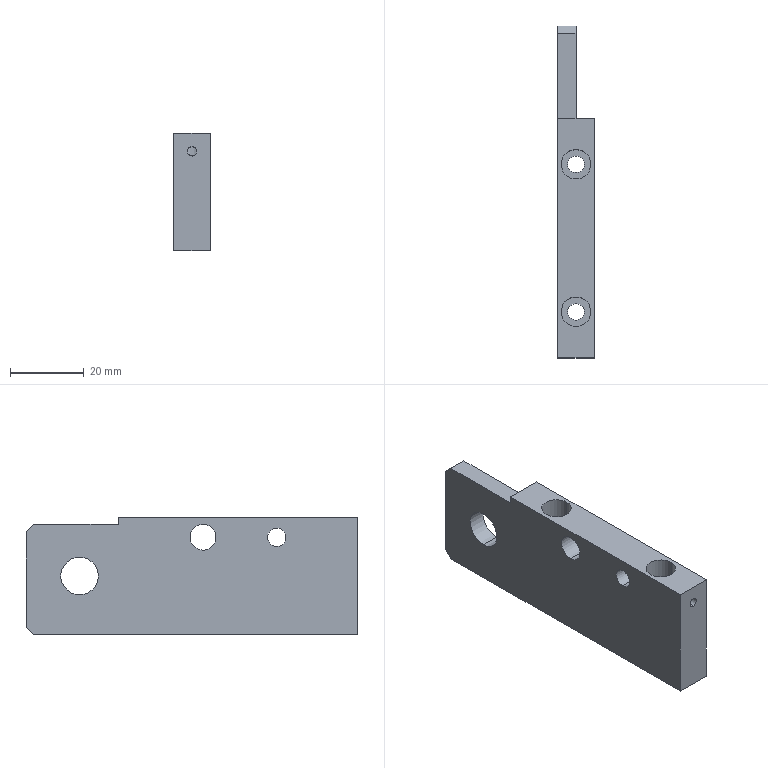Part | STEP file | PN_0065 Mount electronic clip s horizontal manipulator rear end cover | 1 solid | 32 faces | box 10 x 90 x 32 mm | volume 20939 mm3 | cylinder 18 | plane 14 | commonest cylinder face diameters 2.5 x4 4.5 x4 8 x4 5 x2 7 x2 10.2 x2